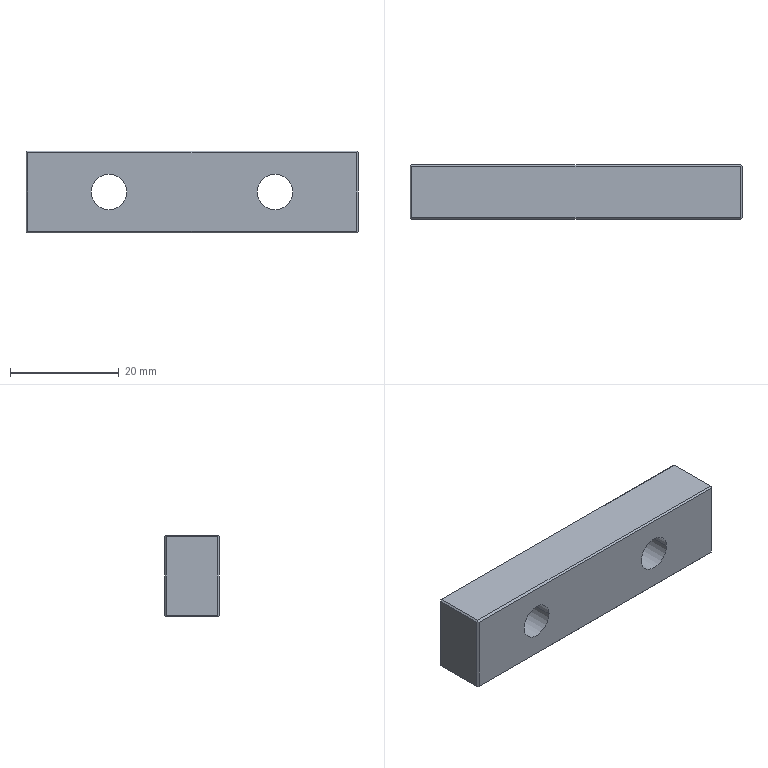Part | NX | 1 solid | 26 faces | box 61 x 10 x 15 mm | volume 8470 mm3 | plane 18 | cylinder 4 | cone 4 | commonest cylinder face diameters 6.5 x4
STEP:
#1=CARTESIAN_POINT('',(-76.,-102.8,-102.3));
#2=VERTEX_POINT('',#1);
#3=CARTESIAN_POINT('',(-76.,-112.2,-102.3));
#4=VERTEX_POINT('',#3);
#5=CARTESIAN_POINT('',(-76.,-107.5,-102.3));
#6=DIRECTION('',(0.,-1.,0.));
#7=VECTOR('',#6,1000.);
#8=LINE('',#5,#7);
#9=EDGE_CURVE('',#2,#4,#8,.T.);
#10=ORIENTED_EDGE('',*,*,#9,.F.);
#11=CARTESIAN_POINT('',(-76.,-102.8,-116.7));
#12=VERTEX_POINT('',#11);
#13=CARTESIAN_POINT('',(-76.,-102.8,-109.5));
#14=DIRECTION('',(0.,0.,-1.));
#15=VECTOR('',#14,1000.);
#16=LINE('',#13,#15);
#17=EDGE_CURVE('',#2,#12,#16,.T.);
#18=ORIENTED_EDGE('',*,*,#17,.T.);
#19=CARTESIAN_POINT('',(-76.,-112.2,-116.7));
#20=VERTEX_POINT('',#19);
#21=CARTESIAN_POINT('',(-76.,-107.5,-116.7));
#22=DIRECTION('',(0.,-1.,0.));
#23=VECTOR('',#22,1000.);
#24=LINE('',#21,#23);
#25=EDGE_CURVE('',#12,#20,#24,.T.);
#26=ORIENTED_EDGE('',*,*,#25,.T.);
#27=CARTESIAN_POINT('',(-76.,-112.2,-109.5));
#28=DIRECTION('',(0.,0.,-1.));
#29=VECTOR('',#28,1000.);
#30=LINE('',#27,#29);
#31=EDGE_CURVE('',#4,#20,#30,.T.);
#32=ORIENTED_EDGE('',*,*,#31,.F.);
#33=EDGE_LOOP('',(#10,#18,#26,#32));
#34=FACE_BOUND('',#33,.T.);
#35=CARTESIAN_POINT('',(-76.,-100.5,-116.5));
#36=DIRECTION('',(-1.,0.,0.));
#37=DIRECTION('',(0.,0.,1.));
#38=AXIS2_PLACEMENT_3D('',#35,#36,#37);
#39=PLANE('',#38);
#40=ADVANCED_FACE('',(#34),#39,.T.);
#41=CARTESIAN_POINT('',(-15.3,-112.2,-117.));
#42=VERTEX_POINT('',#41);
#43=CARTESIAN_POINT('',(-15.3,-102.8,-117.));
#44=VERTEX_POINT('',#43);
#45=CARTESIAN_POINT('',(-15.3,-107.5,-117.));
#46=DIRECTION('',(0.,1.,0.));
#47=VECTOR('',#46,1000.);
#48=LINE('',#45,#47);
#49=EDGE_CURVE('',#42,#44,#48,.T.);
#50=ORIENTED_EDGE('',*,*,#49,.F.);
#51=CARTESIAN_POINT('',(-75.7,-112.2,-117.));
#52=VERTEX_POINT('',#51);
#53=CARTESIAN_POINT('',(-45.5,-112.2,-117.));
#54=DIRECTION('',(-1.,0.,0.));
#55=VECTOR('',#54,1000.);
#56=LINE('',#53,#55);
#57=EDGE_CURVE('',#42,#52,#56,.T.);
#58=ORIENTED_EDGE('',*,*,#57,.T.);
#59=CARTESIAN_POINT('',(-75.7,-102.8,-117.));
#60=VERTEX_POINT('',#59);
#61=CARTESIAN_POINT('',(-75.7,-107.5,-117.));
#62=DIRECTION('',(0.,-1.,0.));
#63=VECTOR('',#62,1000.);
#64=LINE('',#61,#63);
#65=EDGE_CURVE('',#60,#52,#64,.T.);
#66=ORIENTED_EDGE('',*,*,#65,.F.);
#67=CARTESIAN_POINT('',(-45.5,-102.8,-117.));
#68=DIRECTION('',(-1.,0.,0.));
#69=VECTOR('',#68,1000.);
#70=LINE('',#67,#69);
#71=EDGE_CURVE('',#44,#60,#70,.T.);
#72=ORIENTED_EDGE('',*,*,#71,.F.);
#73=EDGE_LOOP('',(#50,#58,#66,#72));
#74=FACE_BOUND('',#73,.T.);
#75=CARTESIAN_POINT('',(-15.,-100.5,-117.));
#76=DIRECTION('',(0.,0.,-1.));
#77=DIRECTION('',(-1.,0.,0.));
#78=AXIS2_PLACEMENT_3D('',#75,#76,#77);
#79=PLANE('',#78);
#80=ADVANCED_FACE('',(#74),#79,.T.);
#81=CARTESIAN_POINT('',(-15.,-102.8,-102.3));
#82=VERTEX_POINT('',#81);
#83=CARTESIAN_POINT('',(-15.,-112.2,-102.3));
#84=VERTEX_POINT('',#83);
#85=CARTESIAN_POINT('',(-15.,-107.5,-102.3));
#86=DIRECTION('',(0.,-1.,0.));
#87=VECTOR('',#86,1000.);
#88=LINE('',#85,#87);
#89=EDGE_CURVE('',#82,#84,#88,.T.);
#90=ORIENTED_EDGE('',*,*,#89,.T.);
#91=CARTESIAN_POINT('',(-15.,-112.2,-116.7));
#92=VERTEX_POINT('',#91);
#93=CARTESIAN_POINT('',(-15.,-112.2,-109.5));
#94=DIRECTION('',(0.,0.,1.));
#95=VECTOR('',#94,1000.);
#96=LINE('',#93,#95);
#97=EDGE_CURVE('',#92,#84,#96,.T.);
#98=ORIENTED_EDGE('',*,*,#97,.F.);
#99=CARTESIAN_POINT('',(-15.,-102.8,-116.7));
#100=VERTEX_POINT('',#99);
#101=CARTESIAN_POINT('',(-15.,-107.5,-116.7));
#102=DIRECTION('',(0.,1.,0.));
#103=VECTOR('',#102,1000.);
#104=LINE('',#101,#103);
#105=EDGE_CURVE('',#92,#100,#104,.T.);
#106=ORIENTED_EDGE('',*,*,#105,.T.);
#107=CARTESIAN_POINT('',(-15.,-102.8,-109.5));
#108=DIRECTION('',(0.,0.,1.));
#109=VECTOR('',#108,1000.);
#110=LINE('',#107,#109);
#111=EDGE_CURVE('',#100,#82,#110,.T.);
#112=ORIENTED_EDGE('',*,*,#111,.T.);
#113=EDGE_LOOP('',(#90,#98,#106,#112));
#114=FACE_BOUND('',#113,.T.);
#115=CARTESIAN_POINT('',(-15.,-100.5,-102.));
#116=DIRECTION('',(1.,0.,0.));
#117=DIRECTION('',(0.,1.,0.));
#118=AXIS2_PLACEMENT_3D('',#115,#116,#117);
#119=PLANE('',#118);
#120=ADVANCED_FACE('',(#114),#119,.T.);
#121=CARTESIAN_POINT('',(-15.3,-102.8,-102.));
#122=VERTEX_POINT('',#121);
#123=CARTESIAN_POINT('',(-75.7,-102.8,-102.));
#124=VERTEX_POINT('',#123);
#125=CARTESIAN_POINT('',(-45.5,-102.8,-102.));
#126=DIRECTION('',(-1.,0.,0.));
#127=VECTOR('',#126,1000.);
#128=LINE('',#125,#127);
#129=EDGE_CURVE('',#122,#124,#128,.T.);
#130=ORIENTED_EDGE('',*,*,#129,.T.);
#131=CARTESIAN_POINT('',(-75.7,-112.2,-102.));
#132=VERTEX_POINT('',#131);
#133=CARTESIAN_POINT('',(-75.7,-107.5,-102.));
#134=DIRECTION('',(0.,-1.,0.));
#135=VECTOR('',#134,1000.);
#136=LINE('',#133,#135);
#137=EDGE_CURVE('',#124,#132,#136,.T.);
#138=ORIENTED_EDGE('',*,*,#137,.T.);
#139=CARTESIAN_POINT('',(-15.3,-112.2,-102.));
#140=VERTEX_POINT('',#139);
#141=CARTESIAN_POINT('',(-45.5,-112.2,-102.));
#142=DIRECTION('',(-1.,0.,0.));
#143=VECTOR('',#142,1000.);
#144=LINE('',#141,#143);
#145=EDGE_CURVE('',#140,#132,#144,.T.);
#146=ORIENTED_EDGE('',*,*,#145,.F.);
#147=CARTESIAN_POINT('',(-15.3,-107.5,-102.));
#148=DIRECTION('',(0.,-1.,0.));
#149=VECTOR('',#148,1000.);
#150=LINE('',#147,#149);
#151=EDGE_CURVE('',#122,#140,#150,.T.);
#152=ORIENTED_EDGE('',*,*,#151,.F.);
#153=EDGE_LOOP('',(#130,#138,#146,#152));
#154=FACE_BOUND('',#153,.T.);
#155=CARTESIAN_POINT('',(-76.,-100.5,-102.));
#156=DIRECTION('',(0.,0.,1.));
#157=DIRECTION('',(0.,-1.,0.));
#158=AXIS2_PLACEMENT_3D('',#155,#156,#157);
#159=PLANE('',#158);
#160=ADVANCED_FACE('',(#154),#159,.T.);
#161=CARTESIAN_POINT('',(-57.5,-102.7,-109.5));
#162=VERTEX_POINT('',#161);
#163=CARTESIAN_POINT('',(-64.,-102.7,-109.5));
#164=VERTEX_POINT('',#163);
#165=CARTESIAN_POINT('',(-60.75,-102.7,-109.5));
#166=DIRECTION('',(0.,1.,0.));
#167=DIRECTION('',(-1.,0.,0.));
#168=AXIS2_PLACEMENT_3D('',#165,#166,#167);
#169=CIRCLE('',#168,3.25);
#170=EDGE_CURVE('',#162,#164,#169,.T.);
#171=ORIENTED_EDGE('',*,*,#170,.T.);
#172=CARTESIAN_POINT('',(-64.,-112.5,-109.5));
#173=VERTEX_POINT('',#172);
#174=CARTESIAN_POINT('',(-64.,-102.5,-109.5));
#175=DIRECTION('',(0.,1.,0.));
#176=VECTOR('',#175,1000.);
#177=LINE('',#174,#176);
#178=EDGE_CURVE('',#164,#173,#177,.F.);
#179=ORIENTED_EDGE('',*,*,#178,.T.);
#180=CARTESIAN_POINT('',(-57.5,-112.5,-109.5));
#181=VERTEX_POINT('',#180);
#182=CARTESIAN_POINT('',(-60.75,-112.5,-109.5));
#183=DIRECTION('',(0.,1.,0.));
#184=DIRECTION('',(-1.,0.,0.));
#185=AXIS2_PLACEMENT_3D('',#182,#183,#184);
#186=CIRCLE('',#185,3.25);
#187=EDGE_CURVE('',#181,#173,#186,.T.);
#188=ORIENTED_EDGE('',*,*,#187,.F.);
#189=CARTESIAN_POINT('',(-57.5,-102.5,-109.5));
#190=DIRECTION('',(0.,1.,0.));
#191=VECTOR('',#190,1000.);
#192=LINE('',#189,#191);
#193=EDGE_CURVE('',#162,#181,#192,.F.);
#194=ORIENTED_EDGE('',*,*,#193,.F.);
#195=EDGE_LOOP('',(#171,#179,#188,#194));
#196=FACE_BOUND('',#195,.T.);
#197=CARTESIAN_POINT('',(-60.75,-102.5,-109.5));
#198=DIRECTION('',(0.,1.,0.));
#199=DIRECTION('',(-1.,0.,0.));
#200=AXIS2_PLACEMENT_3D('',#197,#198,#199);
#201=CYLINDRICAL_SURFACE('',#200,3.25);
#202=ADVANCED_FACE('',(#196),#201,.F.);
#203=ORIENTED_EDGE('',*,*,#170,.F.);
#204=CARTESIAN_POINT('',(-57.3,-102.5,-109.5));
#205=VERTEX_POINT('',#204);
#206=CARTESIAN_POINT('',(-57.5,-102.7,-109.5));
#207=DIRECTION('',(0.7071,0.7071,0.));
#208=VECTOR('',#207,1000.);
#209=LINE('',#206,#208);
#210=EDGE_CURVE('',#205,#162,#209,.F.);
#211=ORIENTED_EDGE('',*,*,#210,.F.);
#212=CARTESIAN_POINT('',(-64.2,-102.5,-109.5));
#213=VERTEX_POINT('',#212);
#214=CARTESIAN_POINT('',(-60.75,-102.5,-109.5));
#215=DIRECTION('',(0.,1.,0.));
#216=DIRECTION('',(-1.,0.,0.));
#217=AXIS2_PLACEMENT_3D('',#214,#215,#216);
#218=CIRCLE('',#217,3.45);
#219=EDGE_CURVE('',#205,#213,#218,.T.);
#220=ORIENTED_EDGE('',*,*,#219,.T.);
#221=CARTESIAN_POINT('',(-64.,-102.7,-109.5));
#222=DIRECTION('',(-0.7071,0.7071,0.));
#223=VECTOR('',#222,1000.);
#224=LINE('',#221,#223);
#225=EDGE_CURVE('',#213,#164,#224,.F.);
#226=ORIENTED_EDGE('',*,*,#225,.T.);
#227=EDGE_LOOP('',(#203,#211,#220,#226));
#228=FACE_BOUND('',#227,.T.);
#229=CARTESIAN_POINT('',(-60.75,-102.7,-109.5));
#230=DIRECTION('',(0.,1.,0.));
#231=DIRECTION('',(-1.,0.,0.));
#232=AXIS2_PLACEMENT_3D('',#229,#230,#231);
#233=CONICAL_SURFACE('',#232,3.25,0.7854);
#234=ADVANCED_FACE('',(#228),#233,.F.);
#235=ORIENTED_EDGE('',*,*,#49,.T.);
#236=CARTESIAN_POINT('',(-15.15,-102.65,-116.85));
#237=VERTEX_POINT('',#236);
#238=CARTESIAN_POINT('',(-45.17,-132.67,-146.87));
#239=DIRECTION('',(-0.5774,-0.5774,-0.5774));
#240=VECTOR('',#239,1000.);
#241=LINE('',#238,#240);
#242=EDGE_CURVE('',#237,#44,#241,.T.);
#243=ORIENTED_EDGE('',*,*,#242,.F.);
#244=CARTESIAN_POINT('',(-45.17,-72.63,-146.87));
#245=DIRECTION('',(0.5774,-0.5774,0.5774));
#246=VECTOR('',#245,1000.);
#247=LINE('',#244,#246);
#248=EDGE_CURVE('',#237,#100,#247,.T.);
#249=ORIENTED_EDGE('',*,*,#248,.T.);
#250=ORIENTED_EDGE('',*,*,#105,.F.);
#251=CARTESIAN_POINT('',(-15.15,-112.35,-116.85));
#252=VERTEX_POINT('',#251);
#253=CARTESIAN_POINT('',(-45.17,-142.37,-146.87));
#254=DIRECTION('',(0.5774,0.5774,0.5774));
#255=VECTOR('',#254,1000.);
#256=LINE('',#253,#255);
#257=EDGE_CURVE('',#252,#92,#256,.T.);
#258=ORIENTED_EDGE('',*,*,#257,.F.);
#259=CARTESIAN_POINT('',(-27.,-100.5,-128.7));
#260=DIRECTION('',(-0.5774,0.5774,-0.5774));
#261=VECTOR('',#260,1000.);
#262=LINE('',#259,#261);
#263=EDGE_CURVE('',#252,#42,#262,.T.);
#264=ORIENTED_EDGE('',*,*,#263,.T.);
#265=EDGE_LOOP('',(#235,#243,#249,#250,#258,#264));
#266=FACE_BOUND('',#265,.T.);
#267=CARTESIAN_POINT('',(-15.15,-107.5,-116.85));
#268=DIRECTION('',(-0.7071,0.,0.7071));
#269=DIRECTION('',(0.,1.,0.));
#270=AXIS2_PLACEMENT_3D('',#267,#268,#269);
#271=PLANE('',#270);
#272=ADVANCED_FACE('',(#266),#271,.F.);
#273=ORIENTED_EDGE('',*,*,#25,.F.);
#274=CARTESIAN_POINT('',(-75.85,-102.65,-116.85));
#275=VERTEX_POINT('',#274);
#276=CARTESIAN_POINT('',(-109.781,-136.581,-82.919));
#277=DIRECTION('',(0.5774,0.5774,-0.5774));
#278=VECTOR('',#277,1000.);
#279=LINE('',#276,#278);
#280=EDGE_CURVE('',#12,#275,#279,.T.);
#281=ORIENTED_EDGE('',*,*,#280,.T.);
#282=CARTESIAN_POINT('',(-78.,-100.5,-114.7));
#283=DIRECTION('',(-0.5774,0.5774,0.5774));
#284=VECTOR('',#283,1000.);
#285=LINE('',#282,#284);
#286=EDGE_CURVE('',#60,#275,#285,.T.);
#287=ORIENTED_EDGE('',*,*,#286,.F.);
#288=ORIENTED_EDGE('',*,*,#65,.T.);
#289=CARTESIAN_POINT('',(-75.85,-112.35,-116.85));
#290=VERTEX_POINT('',#289);
#291=CARTESIAN_POINT('',(-64.,-100.5,-128.7));
#292=DIRECTION('',(0.5774,0.5774,-0.5774));
#293=VECTOR('',#292,1000.);
#294=LINE('',#291,#293);
#295=EDGE_CURVE('',#290,#52,#294,.T.);
#296=ORIENTED_EDGE('',*,*,#295,.F.);
#297=CARTESIAN_POINT('',(-87.7,-100.5,-105.));
#298=DIRECTION('',(-0.5774,0.5774,0.5774));
#299=VECTOR('',#298,1000.);
#300=LINE('',#297,#299);
#301=EDGE_CURVE('',#290,#20,#300,.T.);
#302=ORIENTED_EDGE('',*,*,#301,.T.);
#303=EDGE_LOOP('',(#273,#281,#287,#288,#296,#302));
#304=FACE_BOUND('',#303,.T.);
#305=CARTESIAN_POINT('',(-75.85,-107.5,-116.85));
#306=DIRECTION('',(-0.7071,0.,-0.7071));
#307=DIRECTION('',(-0.7071,0.,0.7071));
#308=AXIS2_PLACEMENT_3D('',#305,#306,#307);
#309=PLANE('',#308);
#310=ADVANCED_FACE('',(#304),#309,.T.);
#311=ORIENTED_EDGE('',*,*,#9,.T.);
#312=CARTESIAN_POINT('',(-75.85,-112.35,-102.15));
#313=VERTEX_POINT('',#312);
#314=CARTESIAN_POINT('',(-87.7,-100.5,-114.));
#315=DIRECTION('',(0.5774,-0.5774,0.5774));
#316=VECTOR('',#315,1000.);
#317=LINE('',#314,#316);
#318=EDGE_CURVE('',#4,#313,#317,.T.);
#319=ORIENTED_EDGE('',*,*,#318,.T.);
#320=CARTESIAN_POINT('',(-64.,-100.5,-90.3));
#321=DIRECTION('',(-0.5774,-0.5774,-0.5774));
#322=VECTOR('',#321,1000.);
#323=LINE('',#320,#322);
#324=EDGE_CURVE('',#132,#313,#323,.T.);
#325=ORIENTED_EDGE('',*,*,#324,.F.);
#326=ORIENTED_EDGE('',*,*,#137,.F.);
#327=CARTESIAN_POINT('',(-75.85,-102.65,-102.15));
#328=VERTEX_POINT('',#327);
#329=CARTESIAN_POINT('',(-56.619,-121.881,-82.919));
#330=DIRECTION('',(-0.5774,0.5774,-0.5774));
#331=VECTOR('',#330,1000.);
#332=LINE('',#329,#331);
#333=EDGE_CURVE('',#124,#328,#332,.T.);
#334=ORIENTED_EDGE('',*,*,#333,.T.);
#335=CARTESIAN_POINT('',(-56.619,-83.419,-82.919));
#336=DIRECTION('',(0.5774,0.5774,0.5774));
#337=VECTOR('',#336,1000.);
#338=LINE('',#335,#337);
#339=EDGE_CURVE('',#2,#328,#338,.T.);
#340=ORIENTED_EDGE('',*,*,#339,.F.);
#341=EDGE_LOOP('',(#311,#319,#325,#326,#334,#340));
#342=FACE_BOUND('',#341,.T.);
#343=CARTESIAN_POINT('',(-75.85,-107.5,-102.15));
#344=DIRECTION('',(0.7071,0.,-0.7071));
#345=DIRECTION('',(0.,-1.,0.));
#346=AXIS2_PLACEMENT_3D('',#343,#344,#345);
#347=PLANE('',#346);
#348=ADVANCED_FACE('',(#342),#347,.F.);
#349=ORIENTED_EDGE('',*,*,#89,.F.);
#350=CARTESIAN_POINT('',(-15.15,-102.65,-102.15));
#351=VERTEX_POINT('',#350);
#352=CARTESIAN_POINT('',(-34.381,-83.419,-82.919));
#353=DIRECTION('',(-0.5774,0.5774,0.5774));
#354=VECTOR('',#353,1000.);
#355=LINE('',#352,#354);
#356=EDGE_CURVE('',#82,#351,#355,.T.);
#357=ORIENTED_EDGE('',*,*,#356,.T.);
#358=CARTESIAN_POINT('',(-34.381,-121.881,-82.919));
#359=DIRECTION('',(-0.5774,-0.5774,0.5774));
#360=VECTOR('',#359,1000.);
#361=LINE('',#358,#360);
#362=EDGE_CURVE('',#351,#122,#361,.T.);
#363=ORIENTED_EDGE('',*,*,#362,.T.);
#364=ORIENTED_EDGE('',*,*,#151,.T.);
#365=CARTESIAN_POINT('',(-15.15,-112.35,-102.15));
#366=VERTEX_POINT('',#365);
#367=CARTESIAN_POINT('',(-34.381,-93.119,-82.919));
#368=DIRECTION('',(-0.5774,0.5774,0.5774));
#369=VECTOR('',#368,1000.);
#370=LINE('',#367,#369);
#371=EDGE_CURVE('',#366,#140,#370,.T.);
#372=ORIENTED_EDGE('',*,*,#371,.F.);
#373=CARTESIAN_POINT('',(-34.381,-131.581,-82.919));
#374=DIRECTION('',(0.5774,0.5774,-0.5774));
#375=VECTOR('',#374,1000.);
#376=LINE('',#373,#375);
#377=EDGE_CURVE('',#366,#84,#376,.T.);
#378=ORIENTED_EDGE('',*,*,#377,.T.);
#379=EDGE_LOOP('',(#349,#357,#363,#364,#372,#378));
#380=FACE_BOUND('',#379,.T.);
#381=CARTESIAN_POINT('',(-15.15,-107.5,-102.15));
#382=DIRECTION('',(0.7071,0.,0.7071));
#383=DIRECTION('',(0.,-1.,0.));
#384=AXIS2_PLACEMENT_3D('',#381,#382,#383);
#385=PLANE('',#384);
#386=ADVANCED_FACE('',(#380),#385,.T.);
#387=ORIENTED_EDGE('',*,*,#178,.F.);
#388=CARTESIAN_POINT('',(-60.75,-102.7,-109.5));
#389=DIRECTION('',(0.,1.,0.));
#390=DIRECTION('',(-1.,0.,0.));
#391=AXIS2_PLACEMENT_3D('',#388,#389,#390);
#392=CIRCLE('',#391,3.25);
#393=EDGE_CURVE('',#164,#162,#392,.T.);
#394=ORIENTED_EDGE('',*,*,#393,.T.);
#395=ORIENTED_EDGE('',*,*,#193,.T.);
#396=CARTESIAN_POINT('',(-60.75,-112.5,-109.5));
#397=DIRECTION('',(0.,1.,0.));
#398=DIRECTION('',(-1.,0.,0.));
#399=AXIS2_PLACEMENT_3D('',#396,#397,#398);
#400=CIRCLE('',#399,3.25);
#401=EDGE_CURVE('',#173,#181,#400,.T.);
#402=ORIENTED_EDGE('',*,*,#401,.F.);
#403=EDGE_LOOP('',(#387,#394,#395,#402));
#404=FACE_BOUND('',#403,.T.);
#405=CARTESIAN_POINT('',(-60.75,-102.5,-109.5));
#406=DIRECTION('',(0.,1.,0.));
#407=DIRECTION('',(-1.,0.,0.));
#408=AXIS2_PLACEMENT_3D('',#405,#406,#407);
#409=CYLINDRICAL_SURFACE('',#408,3.25);
#410=ADVANCED_FACE('',(#404),#409,.F.);
#411=ORIENTED_EDGE('',*,*,#225,.F.);
#412=CARTESIAN_POINT('',(-60.75,-102.5,-109.5));
#413=DIRECTION('',(0.,1.,0.));
#414=DIRECTION('',(-1.,0.,0.));
#415=AXIS2_PLACEMENT_3D('',#412,#413,#414);
#416=CIRCLE('',#415,3.45);
#417=EDGE_CURVE('',#213,#205,#416,.T.);
#418=ORIENTED_EDGE('',*,*,#417,.T.);
#419=ORIENTED_EDGE('',*,*,#210,.T.);
#420=ORIENTED_EDGE('',*,*,#393,.F.);
#421=EDGE_LOOP('',(#411,#418,#419,#420));
#422=FACE_BOUND('',#421,.T.);
#423=CARTESIAN_POINT('',(-60.75,-102.7,-109.5));
#424=DIRECTION('',(0.,1.,0.));
#425=DIRECTION('',(-1.,0.,0.));
#426=AXIS2_PLACEMENT_3D('',#423,#424,#425);
#427=CONICAL_SURFACE('',#426,3.25,0.7854);
#428=ADVANCED_FACE('',(#422),#427,.F.);
#429=CARTESIAN_POINT('',(-15.3,-112.5,-116.7));
#430=VERTEX_POINT('',#429);
#431=CARTESIAN_POINT('',(-15.3,-112.5,-102.3));
#432=VERTEX_POINT('',#431);
#433=CARTESIAN_POINT('',(-15.3,-112.5,-109.5));
#434=DIRECTION('',(0.,0.,1.));
#435=VECTOR('',#434,1000.);
#436=LINE('',#433,#435);
#437=EDGE_CURVE('',#430,#432,#436,.T.);
#438=ORIENTED_EDGE('',*,*,#437,.T.);
#439=CARTESIAN_POINT('',(-75.7,-112.5,-102.3));
#440=VERTEX_POINT('',#439);
#441=CARTESIAN_POINT('',(-45.5,-112.5,-102.3));
#442=DIRECTION('',(-1.,0.,0.));
#443=VECTOR('',#442,1000.);
#444=LINE('',#441,#443);
#445=EDGE_CURVE('',#432,#440,#444,.T.);
#446=ORIENTED_EDGE('',*,*,#445,.T.);
#447=CARTESIAN_POINT('',(-75.7,-112.5,-116.7));
#448=VERTEX_POINT('',#447);
#449=CARTESIAN_POINT('',(-75.7,-112.5,-109.5));
#450=DIRECTION('',(0.,0.,-1.));
#451=VECTOR('',#450,1000.);
#452=LINE('',#449,#451);
#453=EDGE_CURVE('',#440,#448,#452,.T.);
#454=ORIENTED_EDGE('',*,*,#453,.T.);
#455=CARTESIAN_POINT('',(-45.5,-112.5,-116.7));
#456=DIRECTION('',(-1.,0.,0.));
#457=VECTOR('',#456,1000.);
#458=LINE('',#455,#457);
#459=EDGE_CURVE('',#430,#448,#458,.T.);
#460=ORIENTED_EDGE('',*,*,#459,.F.);
#461=EDGE_LOOP('',(#438,#446,#454,#460));
#462=FACE_BOUND('',#461,.T.);
#463=CARTESIAN_POINT('',(-27.,-112.5,-109.5));
#464=VERTEX_POINT('',#463);
#465=CARTESIAN_POINT('',(-33.5,-112.5,-109.5));
#466=VERTEX_POINT('',#465);
#467=CARTESIAN_POINT('',(-30.25,-112.5,-109.5));
#468=DIRECTION('',(0.,1.,0.));
#469=DIRECTION('',(-1.,0.,0.));
#470=AXIS2_PLACEMENT_3D('',#467,#468,#469);
#471=CIRCLE('',#470,3.25);
#472=EDGE_CURVE('',#464,#466,#471,.T.);
#473=ORIENTED_EDGE('',*,*,#472,.T.);
#474=CARTESIAN_POINT('',(-30.25,-112.5,-109.5));
#475=DIRECTION('',(0.,1.,0.));
#476=DIRECTION('',(-1.,0.,0.));
#477=AXIS2_PLACEMENT_3D('',#474,#475,#476);
#478=CIRCLE('',#477,3.25);
#479=EDGE_CURVE('',#466,#464,#478,.T.);
#480=ORIENTED_EDGE('',*,*,#479,.T.);
#481=EDGE_LOOP('',(#473,#480));
#482=FACE_BOUND('',#481,.T.);
#483=ORIENTED_EDGE('',*,*,#187,.T.);
#484=ORIENTED_EDGE('',*,*,#401,.T.);
#485=EDGE_LOOP('',(#483,#484));
#486=FACE_BOUND('',#485,.T.);
#487=CARTESIAN_POINT('',(-45.17,-112.5,-82.919));
#488=DIRECTION('',(0.,1.,0.));
#489=DIRECTION('',(0.,0.,-1.));
#490=AXIS2_PLACEMENT_3D('',#487,#488,#489);
#491=PLANE('',#490);
#492=ADVANCED_FACE('',(#462,#482,#486),#491,.F.);
#493=CARTESIAN_POINT('',(-27.,-102.7,-109.5));
#494=VERTEX_POINT('',#493);
#495=CARTESIAN_POINT('',(-33.5,-102.7,-109.5));
#496=VERTEX_POINT('',#495);
#497=CARTESIAN_POINT('',(-30.25,-102.7,-109.5));
#498=DIRECTION('',(0.,1.,0.));
#499=DIRECTION('',(-1.,0.,0.));
#500=AXIS2_PLACEMENT_3D('',#497,#498,#499);
#501=CIRCLE('',#500,3.25);
#502=EDGE_CURVE('',#494,#496,#501,.T.);
#503=ORIENTED_EDGE('',*,*,#502,.T.);
#504=CARTESIAN_POINT('',(-33.5,-102.5,-109.5));
#505=DIRECTION('',(0.,1.,0.));
#506=VECTOR('',#505,1000.);
#507=LINE('',#504,#506);
#508=EDGE_CURVE('',#496,#466,#507,.F.);
#509=ORIENTED_EDGE('',*,*,#508,.T.);
#510=ORIENTED_EDGE('',*,*,#472,.F.);
#511=CARTESIAN_POINT('',(-27.,-102.5,-109.5));
#512=DIRECTION('',(0.,1.,0.));
#513=VECTOR('',#512,1000.);
#514=LINE('',#511,#513);
#515=EDGE_CURVE('',#494,#464,#514,.F.);
#516=ORIENTED_EDGE('',*,*,#515,.F.);
#517=EDGE_LOOP('',(#503,#509,#510,#516));
#518=FACE_BOUND('',#517,.T.);
#519=CARTESIAN_POINT('',(-30.25,-102.5,-109.5));
#520=DIRECTION('',(0.,1.,0.));
#521=DIRECTION('',(-1.,0.,0.));
#522=AXIS2_PLACEMENT_3D('',#519,#520,#521);
#523=CYLINDRICAL_SURFACE('',#522,3.25);
#524=ADVANCED_FACE('',(#518),#523,.F.);
#525=ORIENTED_EDGE('',*,*,#502,.F.);
#526=CARTESIAN_POINT('',(-26.8,-102.5,-109.5));
#527=VERTEX_POINT('',#526);
#528=CARTESIAN_POINT('',(-27.,-102.7,-109.5));
#529=DIRECTION('',(0.7071,0.7071,0.));
#530=VECTOR('',#529,1000.);
#531=LINE('',#528,#530);
#532=EDGE_CURVE('',#527,#494,#531,.F.);
#533=ORIENTED_EDGE('',*,*,#532,.F.);
#534=CARTESIAN_POINT('',(-33.7,-102.5,-109.5));
#535=VERTEX_POINT('',#534);
#536=CARTESIAN_POINT('',(-30.25,-102.5,-109.5));
#537=DIRECTION('',(0.,1.,0.));
#538=DIRECTION('',(-1.,0.,0.));
#539=AXIS2_PLACEMENT_3D('',#536,#537,#538);
#540=CIRCLE('',#539,3.45);
#541=EDGE_CURVE('',#527,#535,#540,.T.);
#542=ORIENTED_EDGE('',*,*,#541,.T.);
#543=CARTESIAN_POINT('',(-33.5,-102.7,-109.5));
#544=DIRECTION('',(-0.7071,0.7071,0.));
#545=VECTOR('',#544,1000.);
#546=LINE('',#543,#545);
#547=EDGE_CURVE('',#535,#496,#546,.F.);
#548=ORIENTED_EDGE('',*,*,#547,.T.);
#549=EDGE_LOOP('',(#525,#533,#542,#548));
#550=FACE_BOUND('',#549,.T.);
#551=CARTESIAN_POINT('',(-30.25,-102.7,-109.5));
#552=DIRECTION('',(0.,1.,0.));
#553=DIRECTION('',(-1.,0.,0.));
#554=AXIS2_PLACEMENT_3D('',#551,#552,#553);
#555=CONICAL_SURFACE('',#554,3.25,0.7854);
#556=ADVANCED_FACE('',(#550),#555,.F.);
#557=ORIENTED_EDGE('',*,*,#459,.T.);
#558=CARTESIAN_POINT('',(-87.7,-100.5,-128.7));
#559=DIRECTION('',(0.5774,-0.5774,0.5774));
#560=VECTOR('',#559,1000.);
#561=LINE('',#558,#560);
#562=EDGE_CURVE('',#290,#448,#561,.T.);
#563=ORIENTED_EDGE('',*,*,#562,.F.);
#564=ORIENTED_EDGE('',*,*,#295,.T.);
#565=ORIENTED_EDGE('',*,*,#57,.F.);
#566=ORIENTED_EDGE('',*,*,#263,.F.);
#567=CARTESIAN_POINT('',(-3.3,-100.5,-128.7));
#568=DIRECTION('',(0.5774,0.5774,-0.5774));
#569=VECTOR('',#568,1000.);
#570=LINE('',#567,#569);
#571=EDGE_CURVE('',#430,#252,#570,.T.);
#572=ORIENTED_EDGE('',*,*,#571,.F.);
#573=EDGE_LOOP('',(#557,#563,#564,#565,#566,#572));
#574=FACE_BOUND('',#573,.T.);
#575=CARTESIAN_POINT('',(-45.5,-112.35,-116.85));
#576=DIRECTION('',(0.,0.7071,0.7071));
#577=DIRECTION('',(1.,0.,0.));
#578=AXIS2_PLACEMENT_3D('',#575,#576,#577);
#579=PLANE('',#578);
#580=ADVANCED_FACE('',(#574),#579,.F.);
#581=ORIENTED_EDGE('',*,*,#453,.F.);
#582=CARTESIAN_POINT('',(-87.7,-100.5,-90.3));
#583=DIRECTION('',(-0.5774,0.5774,0.5774));
#584=VECTOR('',#583,1000.);
#585=LINE('',#582,#584);
#586=EDGE_CURVE('',#440,#313,#585,.T.);
#587=ORIENTED_EDGE('',*,*,#586,.T.);
#588=ORIENTED_EDGE('',*,*,#318,.F.);
#589=ORIENTED_EDGE('',*,*,#31,.T.);
#590=ORIENTED_EDGE('',*,*,#301,.F.);
#591=ORIENTED_EDGE('',*,*,#562,.T.);
#592=EDGE_LOOP('',(#581,#587,#588,#589,#590,#591));
#593=FACE_BOUND('',#592,.T.);
#594=CARTESIAN_POINT('',(-75.85,-112.35,-109.5));
#595=DIRECTION('',(-0.7071,-0.7071,0.));
#596=DIRECTION('',(-0.7071,0.7071,0.));
#597=AXIS2_PLACEMENT_3D('',#594,#595,#596);
#598=PLANE('',#597);
#599=ADVANCED_FACE('',(#593),#598,.T.);
#600=ORIENTED_EDGE('',*,*,#445,.F.);
#601=CARTESIAN_POINT('',(-3.3,-100.5,-90.3));
#602=DIRECTION('',(0.5774,0.5774,0.5774));
#603=VECTOR('',#602,1000.);
#604=LINE('',#601,#603);
#605=EDGE_CURVE('',#432,#366,#604,.T.);
#606=ORIENTED_EDGE('',*,*,#605,.T.);
#607=ORIENTED_EDGE('',*,*,#371,.T.);
#608=ORIENTED_EDGE('',*,*,#145,.T.);
#609=ORIENTED_EDGE('',*,*,#324,.T.);
#610=ORIENTED_EDGE('',*,*,#586,.F.);
#611=EDGE_LOOP('',(#600,#606,#607,#608,#609,#610));
#612=FACE_BOUND('',#611,.T.);
#613=CARTESIAN_POINT('',(-45.5,-112.35,-102.15));
#614=DIRECTION('',(0.,-0.7071,0.7071));
#615=DIRECTION('',(-1.,0.,0.));
#616=AXIS2_PLACEMENT_3D('',#613,#614,#615);
#617=PLANE('',#616);
#618=ADVANCED_FACE('',(#612),#617,.T.);
#619=ORIENTED_EDGE('',*,*,#437,.F.);
#620=ORIENTED_EDGE('',*,*,#571,.T.);
#621=ORIENTED_EDGE('',*,*,#257,.T.);
#622=ORIENTED_EDGE('',*,*,#97,.T.);
#623=ORIENTED_EDGE('',*,*,#377,.F.);
#624=ORIENTED_EDGE('',*,*,#605,.F.);
#625=EDGE_LOOP('',(#619,#620,#621,#622,#623,#624));
#626=FACE_BOUND('',#625,.T.);
#627=CARTESIAN_POINT('',(-15.15,-112.35,-109.5));
#628=DIRECTION('',(0.7071,-0.7071,0.));
#629=DIRECTION('',(0.,0.,-1.));
#630=AXIS2_PLACEMENT_3D('',#627,#628,#629);
#631=PLANE('',#630);
#632=ADVANCED_FACE('',(#626),#631,.T.);
#633=ORIENTED_EDGE('',*,*,#508,.F.);
#634=CARTESIAN_POINT('',(-30.25,-102.7,-109.5));
#635=DIRECTION('',(0.,1.,0.));
#636=DIRECTION('',(-1.,0.,0.));
#637=AXIS2_PLACEMENT_3D('',#634,#635,#636);
#638=CIRCLE('',#637,3.25);
#639=EDGE_CURVE('',#496,#494,#638,.T.);
#640=ORIENTED_EDGE('',*,*,#639,.T.);
#641=ORIENTED_EDGE('',*,*,#515,.T.);
#642=ORIENTED_EDGE('',*,*,#479,.F.);
#643=EDGE_LOOP('',(#633,#640,#641,#642));
#644=FACE_BOUND('',#643,.T.);
#645=CARTESIAN_POINT('',(-30.25,-102.5,-109.5));
#646=DIRECTION('',(0.,1.,0.));
#647=DIRECTION('',(-1.,0.,0.));
#648=AXIS2_PLACEMENT_3D('',#645,#646,#647);
#649=CYLINDRICAL_SURFACE('',#648,3.25);
#650=ADVANCED_FACE('',(#644),#649,.F.);
#651=ORIENTED_EDGE('',*,*,#547,.F.);
#652=CARTESIAN_POINT('',(-30.25,-102.5,-109.5));
#653=DIRECTION('',(0.,1.,0.));
#654=DIRECTION('',(-1.,0.,0.));
#655=AXIS2_PLACEMENT_3D('',#652,#653,#654);
#656=CIRCLE('',#655,3.45);
#657=EDGE_CURVE('',#535,#527,#656,.T.);
#658=ORIENTED_EDGE('',*,*,#657,.T.);
#659=ORIENTED_EDGE('',*,*,#532,.T.);
#660=ORIENTED_EDGE('',*,*,#639,.F.);
#661=EDGE_LOOP('',(#651,#658,#659,#660));
#662=FACE_BOUND('',#661,.T.);
#663=CARTESIAN_POINT('',(-30.25,-102.7,-109.5));
#664=DIRECTION('',(0.,1.,0.));
#665=DIRECTION('',(-1.,0.,0.));
#666=AXIS2_PLACEMENT_3D('',#663,#664,#665);
#667=CONICAL_SURFACE('',#666,3.25,0.7854);
#668=ADVANCED_FACE('',(#662),#667,.F.);
#669=CARTESIAN_POINT('',(-15.3,-102.5,-102.3));
#670=VERTEX_POINT('',#669);
#671=CARTESIAN_POINT('',(-75.7,-102.5,-102.3));
#672=VERTEX_POINT('',#671);
#673=CARTESIAN_POINT('',(-45.5,-102.5,-102.3));
#674=DIRECTION('',(-1.,0.,0.));
#675=VECTOR('',#674,1000.);
#676=LINE('',#673,#675);
#677=EDGE_CURVE('',#670,#672,#676,.T.);
#678=ORIENTED_EDGE('',*,*,#677,.F.);
#679=CARTESIAN_POINT('',(-15.3,-102.5,-116.7));
#680=VERTEX_POINT('',#679);
#681=CARTESIAN_POINT('',(-15.3,-102.5,-109.5));
#682=DIRECTION('',(0.,0.,1.));
#683=VECTOR('',#682,1000.);
#684=LINE('',#681,#683);
#685=EDGE_CURVE('',#680,#670,#684,.T.);
#686=ORIENTED_EDGE('',*,*,#685,.F.);
#687=CARTESIAN_POINT('',(-75.7,-102.5,-116.7));
#688=VERTEX_POINT('',#687);
#689=CARTESIAN_POINT('',(-45.5,-102.5,-116.7));
#690=DIRECTION('',(-1.,0.,0.));
#691=VECTOR('',#690,1000.);
#692=LINE('',#689,#691);
#693=EDGE_CURVE('',#680,#688,#692,.T.);
#694=ORIENTED_EDGE('',*,*,#693,.T.);
#695=CARTESIAN_POINT('',(-75.7,-102.5,-109.5));
#696=DIRECTION('',(0.,0.,-1.));
#697=VECTOR('',#696,1000.);
#698=LINE('',#695,#697);
#699=EDGE_CURVE('',#672,#688,#698,.T.);
#700=ORIENTED_EDGE('',*,*,#699,.F.);
#701=EDGE_LOOP('',(#678,#686,#694,#700));
#702=FACE_BOUND('',#701,.T.);
#703=ORIENTED_EDGE('',*,*,#219,.F.);
#704=ORIENTED_EDGE('',*,*,#417,.F.);
#705=EDGE_LOOP('',(#703,#704));
#706=FACE_BOUND('',#705,.T.);
#707=ORIENTED_EDGE('',*,*,#541,.F.);
#708=ORIENTED_EDGE('',*,*,#657,.F.);
#709=EDGE_LOOP('',(#707,#708));
#710=FACE_BOUND('',#709,.T.);
#711=CARTESIAN_POINT('',(-45.17,-102.5,-82.919));
#712=DIRECTION('',(0.,1.,0.));
#713=DIRECTION('',(0.,0.,-1.));
#714=AXIS2_PLACEMENT_3D('',#711,#712,#713);
#715=PLANE('',#714);
#716=ADVANCED_FACE('',(#702,#706,#710),#715,.T.);
#717=ORIENTED_EDGE('',*,*,#685,.T.);
#718=CARTESIAN_POINT('',(4.081,-121.881,-82.919));
#719=DIRECTION('',(0.5774,-0.5774,0.5774));
#720=VECTOR('',#719,1000.);
#721=LINE('',#718,#720);
#722=EDGE_CURVE('',#670,#351,#721,.T.);
#723=ORIENTED_EDGE('',*,*,#722,.T.);
#724=ORIENTED_EDGE('',*,*,#356,.F.);
#725=ORIENTED_EDGE('',*,*,#111,.F.);
#726=ORIENTED_EDGE('',*,*,#248,.F.);
#727=CARTESIAN_POINT('',(-45.17,-72.63,-86.83));
#728=DIRECTION('',(0.5774,-0.5774,-0.5774));
#729=VECTOR('',#728,1000.);
#730=LINE('',#727,#729);
#731=EDGE_CURVE('',#680,#237,#730,.T.);
#732=ORIENTED_EDGE('',*,*,#731,.F.);
#733=EDGE_LOOP('',(#717,#723,#724,#725,#726,#732));
#734=FACE_BOUND('',#733,.T.);
#735=CARTESIAN_POINT('',(-15.15,-102.65,-109.5));
#736=DIRECTION('',(-0.7071,-0.7071,0.));
#737=DIRECTION('',(-0.7071,0.7071,0.));
#738=AXIS2_PLACEMENT_3D('',#735,#736,#737);
#739=PLANE('',#738);
#740=ADVANCED_FACE('',(#734),#739,.F.);
#741=ORIENTED_EDGE('',*,*,#693,.F.);
#742=ORIENTED_EDGE('',*,*,#731,.T.);
#743=ORIENTED_EDGE('',*,*,#242,.T.);
#744=ORIENTED_EDGE('',*,*,#71,.T.);
#745=ORIENTED_EDGE('',*,*,#286,.T.);
#746=CARTESIAN_POINT('',(-45.17,-71.97,-86.17));
#747=DIRECTION('',(-0.5774,-0.5774,-0.5774));
#748=VECTOR('',#747,1000.);
#749=LINE('',#746,#748);
#750=EDGE_CURVE('',#688,#275,#749,.T.);
#751=ORIENTED_EDGE('',*,*,#750,.F.);
#752=EDGE_LOOP('',(#741,#742,#743,#744,#745,#751));
#753=FACE_BOUND('',#752,.T.);
#754=CARTESIAN_POINT('',(-45.5,-102.65,-116.85));
#755=DIRECTION('',(0.,0.7071,-0.7071));
#756=DIRECTION('',(-1.,0.,0.));
#757=AXIS2_PLACEMENT_3D('',#754,#755,#756);
#758=PLANE('',#757);
#759=ADVANCED_FACE('',(#753),#758,.T.);
#760=ORIENTED_EDGE('',*,*,#699,.T.);
#761=ORIENTED_EDGE('',*,*,#750,.T.);
#762=ORIENTED_EDGE('',*,*,#280,.F.);
#763=ORIENTED_EDGE('',*,*,#17,.F.);
#764=ORIENTED_EDGE('',*,*,#339,.T.);
#765=CARTESIAN_POINT('',(-95.081,-121.881,-82.919));
#766=DIRECTION('',(0.5774,0.5774,-0.5774));
#767=VECTOR('',#766,1000.);
#768=LINE('',#765,#767);
#769=EDGE_CURVE('',#328,#672,#768,.T.);
#770=ORIENTED_EDGE('',*,*,#769,.T.);
#771=EDGE_LOOP('',(#760,#761,#762,#763,#764,#770));
#772=FACE_BOUND('',#771,.T.);
#773=CARTESIAN_POINT('',(-75.85,-102.65,-109.5));
#774=DIRECTION('',(0.7071,-0.7071,0.));
#775=DIRECTION('',(0.,0.,-1.));
#776=AXIS2_PLACEMENT_3D('',#773,#774,#775);
#777=PLANE('',#776);
#778=ADVANCED_FACE('',(#772),#777,.F.);
#779=ORIENTED_EDGE('',*,*,#677,.T.);
#780=ORIENTED_EDGE('',*,*,#769,.F.);
#781=ORIENTED_EDGE('',*,*,#333,.F.);
#782=ORIENTED_EDGE('',*,*,#129,.F.);
#783=ORIENTED_EDGE('',*,*,#362,.F.);
#784=ORIENTED_EDGE('',*,*,#722,.F.);
#785=EDGE_LOOP('',(#779,#780,#781,#782,#783,#784));
#786=FACE_BOUND('',#785,.T.);
#787=CARTESIAN_POINT('',(-45.5,-102.65,-102.15));
#788=DIRECTION('',(0.,-0.7071,-0.7071));
#789=DIRECTION('',(0.,0.7071,-0.7071));
#790=AXIS2_PLACEMENT_3D('',#787,#788,#789);
#791=PLANE('',#790);
#792=ADVANCED_FACE('',(#786),#791,.F.);
#793=CLOSED_SHELL('',(#40,#80,#120,#160,#202,#234,#272,#310,#348,#386,#410,#428,#492,#524,#556,#580,#599,#618,#632,#650,#668,#716,#740,#759,#778,#792));
#794=MANIFOLD_SOLID_BREP('',#793);
#795=(LENGTH_UNIT()NAMED_UNIT(*)SI_UNIT(.MILLI.,.METRE.));
#796=UNCERTAINTY_MEASURE_WITH_UNIT(LENGTH_MEASURE(0.00001),#795,'','');
#797=(NAMED_UNIT(*)PLANE_ANGLE_UNIT()SI_UNIT($,.RADIAN.));
#798=(NAMED_UNIT(*)SI_UNIT($,.STERADIAN.)SOLID_ANGLE_UNIT());
#799=(GEOMETRIC_REPRESENTATION_CONTEXT(3)GLOBAL_UNCERTAINTY_ASSIGNED_CONTEXT((#796))GLOBAL_UNIT_ASSIGNED_CONTEXT((#795,#797,#798))REPRESENTATION_CONTEXT('',''));
#800=ADVANCED_BREP_SHAPE_REPRESENTATION('',(#794),#799);